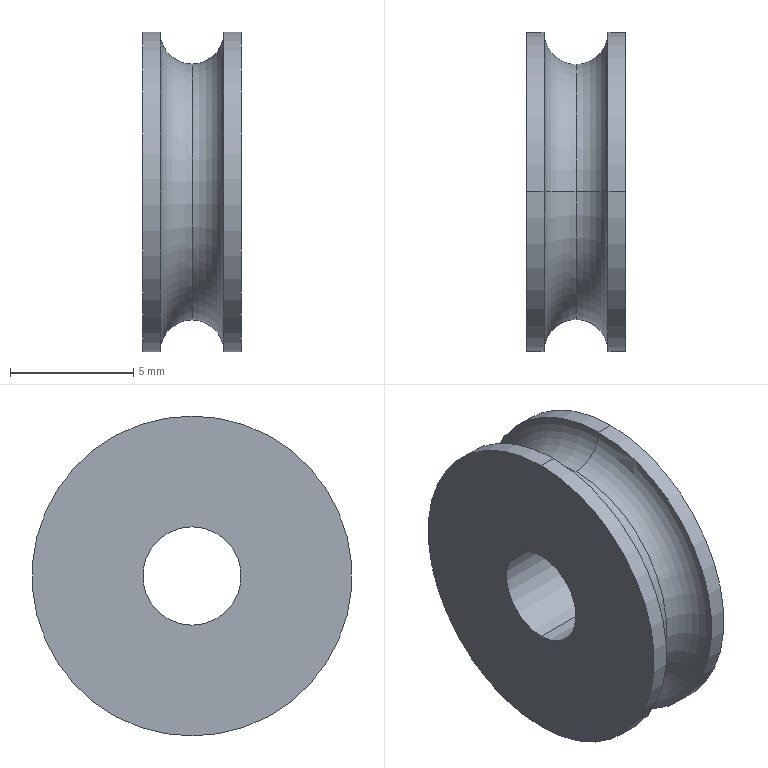Part | SolidWorks | features Revolution 1 | 1 solid | 12 faces | box 4 x 13 x 13 mm | volume 381.449 mm3 | cylinder 6 | torus 4 | plane 2 | commonest cylinder face diameters 13 x4 4 x2
STEP:
#1=CARTESIAN_POINT('',(0.7,0.,6.5));
#2=VERTEX_POINT('',#1);
#3=CARTESIAN_POINT('',(2.,0.,5.2));
#4=VERTEX_POINT('',#3);
#5=CARTESIAN_POINT('',(2.,0.,6.5));
#6=DIRECTION('',(0.,-1.,0.));
#7=DIRECTION('',(0.,0.,-1.));
#8=AXIS2_PLACEMENT_3D('',#5,#6,#7);
#9=CIRCLE('',#8,1.3);
#10=EDGE_CURVE('',#2,#4,#9,.T.);
#11=ORIENTED_EDGE('',*,*,#10,.T.);
#12=CARTESIAN_POINT('',(2.,0.,-5.2));
#13=VERTEX_POINT('',#12);
#14=CARTESIAN_POINT('',(2.,0.,0.));
#15=DIRECTION('',(-1.,0.,0.));
#16=DIRECTION('',(0.,0.,1.));
#17=AXIS2_PLACEMENT_3D('',#14,#15,#16);
#18=CIRCLE('',#17,5.2);
#19=EDGE_CURVE('',#4,#13,#18,.T.);
#20=ORIENTED_EDGE('',*,*,#19,.T.);
#21=CARTESIAN_POINT('',(0.7,0.,-6.5));
#22=VERTEX_POINT('',#21);
#23=CARTESIAN_POINT('',(2.,0.,-6.5));
#24=DIRECTION('',(0.,1.,0.));
#25=DIRECTION('',(0.,0.,1.));
#26=AXIS2_PLACEMENT_3D('',#23,#24,#25);
#27=CIRCLE('',#26,1.3);
#28=EDGE_CURVE('',#22,#13,#27,.T.);
#29=ORIENTED_EDGE('',*,*,#28,.F.);
#30=CARTESIAN_POINT('',(0.7,0.,0.));
#31=DIRECTION('',(-1.,0.,0.));
#32=DIRECTION('',(0.,0.,1.));
#33=AXIS2_PLACEMENT_3D('',#30,#31,#32);
#34=CIRCLE('',#33,6.5);
#35=EDGE_CURVE('',#2,#22,#34,.T.);
#36=ORIENTED_EDGE('',*,*,#35,.F.);
#37=EDGE_LOOP('',(#11,#20,#29,#36));
#38=FACE_OUTER_BOUND('',#37,.T.);
#39=CARTESIAN_POINT('',(2.,0.,0.));
#40=DIRECTION('',(-1.,0.,0.));
#41=DIRECTION('',(0.,0.,1.));
#42=AXIS2_PLACEMENT_3D('',#39,#40,#41);
#43=TOROIDAL_SURFACE('',#42,6.5,1.3);
#44=ADVANCED_FACE('',(#38),#43,.F.);
#45=ORIENTED_EDGE('',*,*,#28,.T.);
#46=CARTESIAN_POINT('',(2.,0.,0.));
#47=DIRECTION('',(-1.,0.,0.));
#48=DIRECTION('',(0.,0.,1.));
#49=AXIS2_PLACEMENT_3D('',#46,#47,#48);
#50=CIRCLE('',#49,5.2);
#51=EDGE_CURVE('',#13,#4,#50,.T.);
#52=ORIENTED_EDGE('',*,*,#51,.T.);
#53=ORIENTED_EDGE('',*,*,#10,.F.);
#54=CARTESIAN_POINT('',(0.7,0.,0.));
#55=DIRECTION('',(-1.,0.,0.));
#56=DIRECTION('',(0.,0.,1.));
#57=AXIS2_PLACEMENT_3D('',#54,#55,#56);
#58=CIRCLE('',#57,6.5);
#59=EDGE_CURVE('',#22,#2,#58,.T.);
#60=ORIENTED_EDGE('',*,*,#59,.F.);
#61=EDGE_LOOP('',(#45,#52,#53,#60));
#62=FACE_OUTER_BOUND('',#61,.T.);
#63=CARTESIAN_POINT('',(2.,0.,0.));
#64=DIRECTION('',(-1.,0.,0.));
#65=DIRECTION('',(0.,0.,1.));
#66=AXIS2_PLACEMENT_3D('',#63,#64,#65);
#67=TOROIDAL_SURFACE('',#66,6.5,1.3);
#68=ADVANCED_FACE('',(#62),#67,.F.);
#69=ORIENTED_EDGE('',*,*,#35,.T.);
#70=CARTESIAN_POINT('',(0.,0.,-6.5));
#71=VERTEX_POINT('',#70);
#72=CARTESIAN_POINT('',(0.,0.,-6.5));
#73=DIRECTION('',(-1.,0.,0.));
#74=VECTOR('',#73,1000.);
#75=LINE('',#72,#74);
#76=EDGE_CURVE('',#22,#71,#75,.T.);
#77=ORIENTED_EDGE('',*,*,#76,.T.);
#78=CARTESIAN_POINT('',(0.,0.,6.5));
#79=VERTEX_POINT('',#78);
#80=CARTESIAN_POINT('',(0.,0.,0.));
#81=DIRECTION('',(-1.,0.,0.));
#82=DIRECTION('',(0.,0.,1.));
#83=AXIS2_PLACEMENT_3D('',#80,#81,#82);
#84=CIRCLE('',#83,6.5);
#85=EDGE_CURVE('',#79,#71,#84,.T.);
#86=ORIENTED_EDGE('',*,*,#85,.F.);
#87=CARTESIAN_POINT('',(0.,0.,6.5));
#88=DIRECTION('',(-1.,0.,0.));
#89=VECTOR('',#88,1000.);
#90=LINE('',#87,#89);
#91=EDGE_CURVE('',#2,#79,#90,.T.);
#92=ORIENTED_EDGE('',*,*,#91,.F.);
#93=EDGE_LOOP('',(#69,#77,#86,#92));
#94=FACE_OUTER_BOUND('',#93,.T.);
#95=CARTESIAN_POINT('',(0.,0.,0.));
#96=DIRECTION('',(-1.,0.,0.));
#97=DIRECTION('',(0.,0.,1.));
#98=AXIS2_PLACEMENT_3D('',#95,#96,#97);
#99=CYLINDRICAL_SURFACE('',#98,6.5);
#100=ADVANCED_FACE('',(#94),#99,.T.);
#101=ORIENTED_EDGE('',*,*,#51,.F.);
#102=CARTESIAN_POINT('',(3.3,0.,-6.5));
#103=VERTEX_POINT('',#102);
#104=CARTESIAN_POINT('',(2.,0.,-6.5));
#105=DIRECTION('',(0.,1.,0.));
#106=DIRECTION('',(0.,0.,1.));
#107=AXIS2_PLACEMENT_3D('',#104,#105,#106);
#108=CIRCLE('',#107,1.3);
#109=EDGE_CURVE('',#13,#103,#108,.T.);
#110=ORIENTED_EDGE('',*,*,#109,.T.);
#111=CARTESIAN_POINT('',(3.3,0.,6.5));
#112=VERTEX_POINT('',#111);
#113=CARTESIAN_POINT('',(3.3,0.,0.));
#114=DIRECTION('',(-1.,0.,0.));
#115=DIRECTION('',(0.,0.,1.));
#116=AXIS2_PLACEMENT_3D('',#113,#114,#115);
#117=CIRCLE('',#116,6.5);
#118=EDGE_CURVE('',#103,#112,#117,.T.);
#119=ORIENTED_EDGE('',*,*,#118,.T.);
#120=CARTESIAN_POINT('',(2.,0.,6.5));
#121=DIRECTION('',(0.,-1.,0.));
#122=DIRECTION('',(0.,0.,-1.));
#123=AXIS2_PLACEMENT_3D('',#120,#121,#122);
#124=CIRCLE('',#123,1.3);
#125=EDGE_CURVE('',#4,#112,#124,.T.);
#126=ORIENTED_EDGE('',*,*,#125,.F.);
#127=EDGE_LOOP('',(#101,#110,#119,#126));
#128=FACE_OUTER_BOUND('',#127,.T.);
#129=CARTESIAN_POINT('',(2.,0.,0.));
#130=DIRECTION('',(-1.,0.,0.));
#131=DIRECTION('',(0.,0.,1.));
#132=AXIS2_PLACEMENT_3D('',#129,#130,#131);
#133=TOROIDAL_SURFACE('',#132,6.5,1.3);
#134=ADVANCED_FACE('',(#128),#133,.F.);
#135=CARTESIAN_POINT('',(4.,0.,6.5));
#136=VERTEX_POINT('',#135);
#137=CARTESIAN_POINT('',(4.,0.,-6.5));
#138=VERTEX_POINT('',#137);
#139=CARTESIAN_POINT('',(4.,0.,0.));
#140=DIRECTION('',(-1.,0.,0.));
#141=DIRECTION('',(0.,0.,1.));
#142=AXIS2_PLACEMENT_3D('',#139,#140,#141);
#143=CIRCLE('',#142,6.5);
#144=EDGE_CURVE('',#136,#138,#143,.T.);
#145=ORIENTED_EDGE('',*,*,#144,.T.);
#146=CARTESIAN_POINT('',(0.,0.,-6.5));
#147=DIRECTION('',(-1.,0.,0.));
#148=VECTOR('',#147,1000.);
#149=LINE('',#146,#148);
#150=EDGE_CURVE('',#138,#103,#149,.T.);
#151=ORIENTED_EDGE('',*,*,#150,.T.);
#152=CARTESIAN_POINT('',(3.3,0.,0.));
#153=DIRECTION('',(-1.,0.,0.));
#154=DIRECTION('',(0.,0.,1.));
#155=AXIS2_PLACEMENT_3D('',#152,#153,#154);
#156=CIRCLE('',#155,6.5);
#157=EDGE_CURVE('',#112,#103,#156,.T.);
#158=ORIENTED_EDGE('',*,*,#157,.F.);
#159=CARTESIAN_POINT('',(0.,0.,6.5));
#160=DIRECTION('',(-1.,0.,0.));
#161=VECTOR('',#160,1000.);
#162=LINE('',#159,#161);
#163=EDGE_CURVE('',#136,#112,#162,.T.);
#164=ORIENTED_EDGE('',*,*,#163,.F.);
#165=EDGE_LOOP('',(#145,#151,#158,#164));
#166=FACE_OUTER_BOUND('',#165,.T.);
#167=CARTESIAN_POINT('',(0.,0.,0.));
#168=DIRECTION('',(-1.,0.,0.));
#169=DIRECTION('',(0.,0.,1.));
#170=AXIS2_PLACEMENT_3D('',#167,#168,#169);
#171=CYLINDRICAL_SURFACE('',#170,6.5);
#172=ADVANCED_FACE('',(#166),#171,.T.);
#173=CARTESIAN_POINT('',(4.,0.,-2.));
#174=VERTEX_POINT('',#173);
#175=CARTESIAN_POINT('',(4.,0.,2.));
#176=VERTEX_POINT('',#175);
#177=CARTESIAN_POINT('',(4.,0.,0.));
#178=DIRECTION('',(-1.,0.,0.));
#179=DIRECTION('',(0.,0.,1.));
#180=AXIS2_PLACEMENT_3D('',#177,#178,#179);
#181=CIRCLE('',#180,2.);
#182=EDGE_CURVE('',#174,#176,#181,.T.);
#183=ORIENTED_EDGE('',*,*,#182,.F.);
#184=CARTESIAN_POINT('',(0.,0.,-2.));
#185=VERTEX_POINT('',#184);
#186=CARTESIAN_POINT('',(0.,0.,-2.));
#187=DIRECTION('',(-1.,0.,0.));
#188=VECTOR('',#187,1000.);
#189=LINE('',#186,#188);
#190=EDGE_CURVE('',#174,#185,#189,.T.);
#191=ORIENTED_EDGE('',*,*,#190,.T.);
#192=CARTESIAN_POINT('',(0.,0.,2.));
#193=VERTEX_POINT('',#192);
#194=CARTESIAN_POINT('',(0.,0.,0.));
#195=DIRECTION('',(-1.,0.,0.));
#196=DIRECTION('',(0.,0.,1.));
#197=AXIS2_PLACEMENT_3D('',#194,#195,#196);
#198=CIRCLE('',#197,2.);
#199=EDGE_CURVE('',#185,#193,#198,.T.);
#200=ORIENTED_EDGE('',*,*,#199,.T.);
#201=CARTESIAN_POINT('',(0.,0.,2.));
#202=DIRECTION('',(-1.,0.,0.));
#203=VECTOR('',#202,1000.);
#204=LINE('',#201,#203);
#205=EDGE_CURVE('',#176,#193,#204,.T.);
#206=ORIENTED_EDGE('',*,*,#205,.F.);
#207=EDGE_LOOP('',(#183,#191,#200,#206));
#208=FACE_OUTER_BOUND('',#207,.T.);
#209=CARTESIAN_POINT('',(0.,0.,0.));
#210=DIRECTION('',(-1.,0.,0.));
#211=DIRECTION('',(0.,0.,1.));
#212=AXIS2_PLACEMENT_3D('',#209,#210,#211);
#213=CYLINDRICAL_SURFACE('',#212,2.);
#214=ADVANCED_FACE('',(#208),#213,.F.);
#215=CARTESIAN_POINT('',(0.,0.,0.));
#216=DIRECTION('',(-1.,0.,0.));
#217=DIRECTION('',(0.,0.,1.));
#218=AXIS2_PLACEMENT_3D('',#215,#216,#217);
#219=CIRCLE('',#218,2.);
#220=EDGE_CURVE('',#193,#185,#219,.T.);
#221=ORIENTED_EDGE('',*,*,#220,.F.);
#222=ORIENTED_EDGE('',*,*,#199,.F.);
#223=EDGE_LOOP('',(#221,#222));
#224=FACE_BOUND('',#223,.T.);
#225=ORIENTED_EDGE('',*,*,#85,.T.);
#226=CARTESIAN_POINT('',(0.,0.,0.));
#227=DIRECTION('',(-1.,0.,0.));
#228=DIRECTION('',(0.,0.,1.));
#229=AXIS2_PLACEMENT_3D('',#226,#227,#228);
#230=CIRCLE('',#229,6.5);
#231=EDGE_CURVE('',#71,#79,#230,.T.);
#232=ORIENTED_EDGE('',*,*,#231,.T.);
#233=EDGE_LOOP('',(#225,#232));
#234=FACE_OUTER_BOUND('',#233,.T.);
#235=CARTESIAN_POINT('',(0.,0.,-2.));
#236=DIRECTION('',(1.,0.,0.));
#237=DIRECTION('',(0.,0.,-1.));
#238=AXIS2_PLACEMENT_3D('',#235,#236,#237);
#239=PLANE('',#238);
#240=ADVANCED_FACE('',(#224,#234),#239,.F.);
#241=ORIENTED_EDGE('',*,*,#190,.F.);
#242=CARTESIAN_POINT('',(4.,0.,0.));
#243=DIRECTION('',(-1.,0.,0.));
#244=DIRECTION('',(0.,0.,1.));
#245=AXIS2_PLACEMENT_3D('',#242,#243,#244);
#246=CIRCLE('',#245,2.);
#247=EDGE_CURVE('',#176,#174,#246,.T.);
#248=ORIENTED_EDGE('',*,*,#247,.F.);
#249=ORIENTED_EDGE('',*,*,#205,.T.);
#250=ORIENTED_EDGE('',*,*,#220,.T.);
#251=EDGE_LOOP('',(#241,#248,#249,#250));
#252=FACE_OUTER_BOUND('',#251,.T.);
#253=CARTESIAN_POINT('',(0.,0.,0.));
#254=DIRECTION('',(-1.,0.,0.));
#255=DIRECTION('',(0.,0.,1.));
#256=AXIS2_PLACEMENT_3D('',#253,#254,#255);
#257=CYLINDRICAL_SURFACE('',#256,2.);
#258=ADVANCED_FACE('',(#252),#257,.F.);
#259=ORIENTED_EDGE('',*,*,#144,.F.);
#260=CARTESIAN_POINT('',(4.,0.,0.));
#261=DIRECTION('',(-1.,0.,0.));
#262=DIRECTION('',(0.,0.,1.));
#263=AXIS2_PLACEMENT_3D('',#260,#261,#262);
#264=CIRCLE('',#263,6.5);
#265=EDGE_CURVE('',#138,#136,#264,.T.);
#266=ORIENTED_EDGE('',*,*,#265,.F.);
#267=EDGE_LOOP('',(#259,#266));
#268=FACE_OUTER_BOUND('',#267,.T.);
#269=ORIENTED_EDGE('',*,*,#247,.T.);
#270=ORIENTED_EDGE('',*,*,#182,.T.);
#271=EDGE_LOOP('',(#269,#270));
#272=FACE_BOUND('',#271,.T.);
#273=CARTESIAN_POINT('',(4.,0.,-2.));
#274=DIRECTION('',(-1.,0.,0.));
#275=DIRECTION('',(0.,0.,1.));
#276=AXIS2_PLACEMENT_3D('',#273,#274,#275);
#277=PLANE('',#276);
#278=ADVANCED_FACE('',(#268,#272),#277,.F.);
#279=ORIENTED_EDGE('',*,*,#150,.F.);
#280=ORIENTED_EDGE('',*,*,#265,.T.);
#281=ORIENTED_EDGE('',*,*,#163,.T.);
#282=ORIENTED_EDGE('',*,*,#118,.F.);
#283=EDGE_LOOP('',(#279,#280,#281,#282));
#284=FACE_OUTER_BOUND('',#283,.T.);
#285=CARTESIAN_POINT('',(0.,0.,0.));
#286=DIRECTION('',(-1.,0.,0.));
#287=DIRECTION('',(0.,0.,1.));
#288=AXIS2_PLACEMENT_3D('',#285,#286,#287);
#289=CYLINDRICAL_SURFACE('',#288,6.5);
#290=ADVANCED_FACE('',(#284),#289,.T.);
#291=ORIENTED_EDGE('',*,*,#19,.F.);
#292=ORIENTED_EDGE('',*,*,#125,.T.);
#293=ORIENTED_EDGE('',*,*,#157,.T.);
#294=ORIENTED_EDGE('',*,*,#109,.F.);
#295=EDGE_LOOP('',(#291,#292,#293,#294));
#296=FACE_OUTER_BOUND('',#295,.T.);
#297=CARTESIAN_POINT('',(2.,0.,0.));
#298=DIRECTION('',(-1.,0.,0.));
#299=DIRECTION('',(0.,0.,1.));
#300=AXIS2_PLACEMENT_3D('',#297,#298,#299);
#301=TOROIDAL_SURFACE('',#300,6.5,1.3);
#302=ADVANCED_FACE('',(#296),#301,.F.);
#303=ORIENTED_EDGE('',*,*,#76,.F.);
#304=ORIENTED_EDGE('',*,*,#59,.T.);
#305=ORIENTED_EDGE('',*,*,#91,.T.);
#306=ORIENTED_EDGE('',*,*,#231,.F.);
#307=EDGE_LOOP('',(#303,#304,#305,#306));
#308=FACE_OUTER_BOUND('',#307,.T.);
#309=CARTESIAN_POINT('',(0.,0.,0.));
#310=DIRECTION('',(-1.,0.,0.));
#311=DIRECTION('',(0.,0.,1.));
#312=AXIS2_PLACEMENT_3D('',#309,#310,#311);
#313=CYLINDRICAL_SURFACE('',#312,6.5);
#314=ADVANCED_FACE('',(#308),#313,.T.);
#315=CLOSED_SHELL('',(#44,#68,#100,#134,#172,#214,#240,#258,#278,#290,#302,#314));
#316=MANIFOLD_SOLID_BREP('',#315);
#317=CARTESIAN_POINT('',(0.,0.,0.));
#318=DIRECTION('',(0.,0.,1.));
#319=DIRECTION('',(1.,0.,0.));
#320=AXIS2_PLACEMENT_3D('',#317,#318,#319);
#321=(LENGTH_UNIT()NAMED_UNIT(*)SI_UNIT(.MILLI.,.METRE.));
#322=UNCERTAINTY_MEASURE_WITH_UNIT(LENGTH_MEASURE(0.00001),#321,'','');
#323=(NAMED_UNIT(*)PLANE_ANGLE_UNIT()SI_UNIT($,.RADIAN.));
#324=(NAMED_UNIT(*)SI_UNIT($,.STERADIAN.)SOLID_ANGLE_UNIT());
#325=(GEOMETRIC_REPRESENTATION_CONTEXT(3)GLOBAL_UNCERTAINTY_ASSIGNED_CONTEXT((#322))GLOBAL_UNIT_ASSIGNED_CONTEXT((#321,#323,#324))REPRESENTATION_CONTEXT('',''));
#326=ADVANCED_BREP_SHAPE_REPRESENTATION('',(#316,#320),#325);